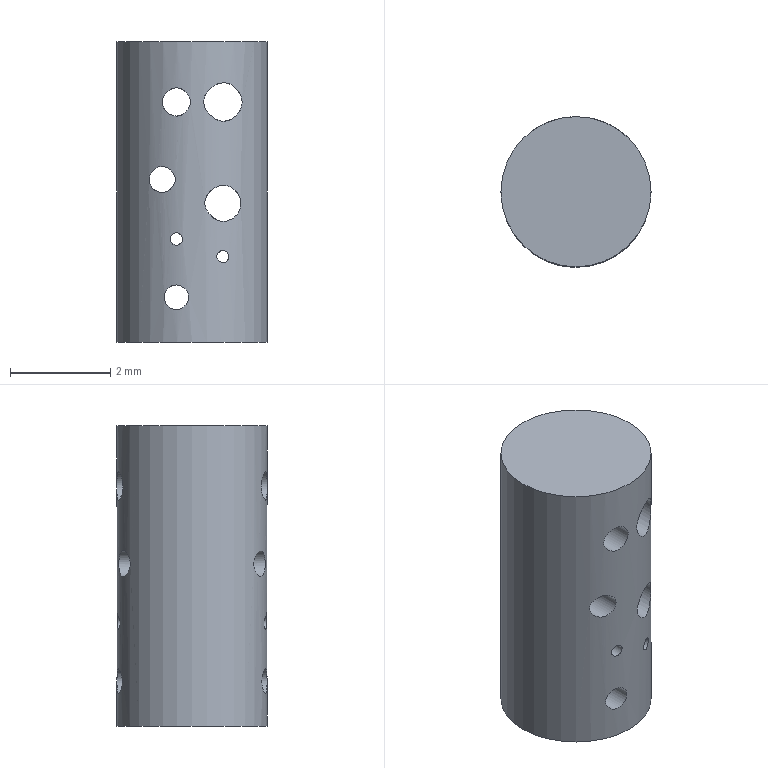Part | NX | features DATUM_CSYS 2, CYLINDER 1, EXTRUDE 1, SKETCH 1 | 1 solid | 10 faces | box 3 x 3 x 6 mm | volume 37.933 mm3 | cylinder 8 | plane 2 | commonest cylinder face diameters 0.245 x1 0.249 x1 0.497 x1 0.522 x1 0.565 x1 0.724 x1